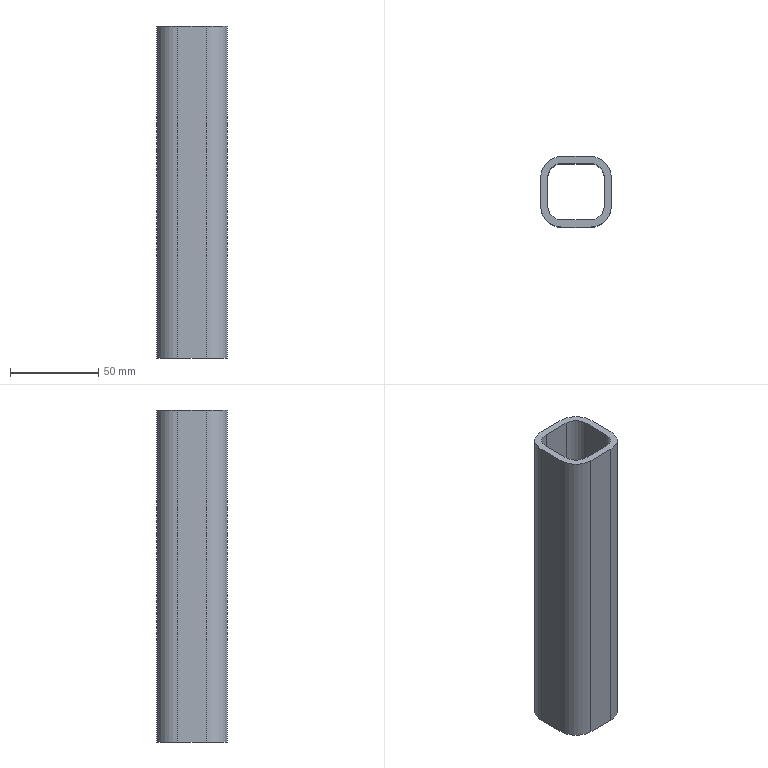Part | SolidWorks | features BaseBody 1 | 1 solid | 18 faces | box 40 x 40 x 188 mm | volume 95378 mm3 | plane 10 | cylinder 8 | commonest cylinder face diameters 16 x4 24 x4
STEP:
#1=CARTESIAN_POINT('',(8.,-20.,0.));
#2=VERTEX_POINT('',#1);
#3=CARTESIAN_POINT('',(20.,-8.,0.));
#4=VERTEX_POINT('',#3);
#5=CARTESIAN_POINT('',(8.,-8.,0.));
#6=DIRECTION('',(0.,0.,1.));
#7=DIRECTION('',(1.,0.,0.));
#8=AXIS2_PLACEMENT_3D('',#5,#6,#7);
#9=CIRCLE('',#8,12.);
#10=EDGE_CURVE('',#2,#4,#9,.T.);
#11=ORIENTED_EDGE('',*,*,#10,.T.);
#12=CARTESIAN_POINT('',(20.,-8.,188.));
#13=VERTEX_POINT('',#12);
#14=CARTESIAN_POINT('',(20.,-8.,0.));
#15=DIRECTION('',(0.,0.,1.));
#16=VECTOR('',#15,1000.);
#17=LINE('',#14,#16);
#18=EDGE_CURVE('',#4,#13,#17,.T.);
#19=ORIENTED_EDGE('',*,*,#18,.T.);
#20=CARTESIAN_POINT('',(8.,-20.,188.));
#21=VERTEX_POINT('',#20);
#22=CARTESIAN_POINT('',(8.,-8.,188.));
#23=DIRECTION('',(0.,0.,-1.));
#24=DIRECTION('',(1.,0.,0.));
#25=AXIS2_PLACEMENT_3D('',#22,#23,#24);
#26=CIRCLE('',#25,12.);
#27=EDGE_CURVE('',#13,#21,#26,.T.);
#28=ORIENTED_EDGE('',*,*,#27,.T.);
#29=CARTESIAN_POINT('',(8.,-20.,0.));
#30=DIRECTION('',(0.,0.,-1.));
#31=VECTOR('',#30,1000.);
#32=LINE('',#29,#31);
#33=EDGE_CURVE('',#21,#2,#32,.T.);
#34=ORIENTED_EDGE('',*,*,#33,.T.);
#35=EDGE_LOOP('',(#11,#19,#28,#34));
#36=FACE_OUTER_BOUND('',#35,.T.);
#37=CARTESIAN_POINT('',(8.,-8.,0.));
#38=DIRECTION('',(0.,0.,1.));
#39=DIRECTION('',(1.,0.,0.));
#40=AXIS2_PLACEMENT_3D('',#37,#38,#39);
#41=CYLINDRICAL_SURFACE('',#40,12.);
#42=ADVANCED_FACE('',(#36),#41,.T.);
#43=CARTESIAN_POINT('',(20.,8.,0.));
#44=VERTEX_POINT('',#43);
#45=CARTESIAN_POINT('',(20.,8.,0.));
#46=DIRECTION('',(0.,1.,0.));
#47=VECTOR('',#46,1000.);
#48=LINE('',#45,#47);
#49=EDGE_CURVE('',#4,#44,#48,.T.);
#50=ORIENTED_EDGE('',*,*,#49,.T.);
#51=CARTESIAN_POINT('',(20.,8.,188.));
#52=VERTEX_POINT('',#51);
#53=CARTESIAN_POINT('',(20.,8.,0.));
#54=DIRECTION('',(0.,0.,1.));
#55=VECTOR('',#54,1000.);
#56=LINE('',#53,#55);
#57=EDGE_CURVE('',#44,#52,#56,.T.);
#58=ORIENTED_EDGE('',*,*,#57,.T.);
#59=CARTESIAN_POINT('',(20.,8.,188.));
#60=DIRECTION('',(0.,-1.,0.));
#61=VECTOR('',#60,1000.);
#62=LINE('',#59,#61);
#63=EDGE_CURVE('',#52,#13,#62,.T.);
#64=ORIENTED_EDGE('',*,*,#63,.T.);
#65=ORIENTED_EDGE('',*,*,#18,.F.);
#66=EDGE_LOOP('',(#50,#58,#64,#65));
#67=FACE_OUTER_BOUND('',#66,.T.);
#68=CARTESIAN_POINT('',(20.,8.,0.));
#69=DIRECTION('',(1.,0.,0.));
#70=DIRECTION('',(0.,1.,0.));
#71=AXIS2_PLACEMENT_3D('',#68,#69,#70);
#72=PLANE('',#71);
#73=ADVANCED_FACE('',(#67),#72,.T.);
#74=CARTESIAN_POINT('',(-16.,8.,0.));
#75=VERTEX_POINT('',#74);
#76=CARTESIAN_POINT('',(-8.,16.,0.));
#77=VERTEX_POINT('',#76);
#78=CARTESIAN_POINT('',(-8.,8.,0.));
#79=DIRECTION('',(0.,0.,-1.));
#80=DIRECTION('',(1.,0.,0.));
#81=AXIS2_PLACEMENT_3D('',#78,#79,#80);
#82=CIRCLE('',#81,8.);
#83=EDGE_CURVE('',#75,#77,#82,.T.);
#84=ORIENTED_EDGE('',*,*,#83,.F.);
#85=CARTESIAN_POINT('',(-16.,-8.,0.));
#86=VERTEX_POINT('',#85);
#87=CARTESIAN_POINT('',(-16.,0.,0.));
#88=DIRECTION('',(0.,1.,0.));
#89=VECTOR('',#88,1000.);
#90=LINE('',#87,#89);
#91=EDGE_CURVE('',#86,#75,#90,.T.);
#92=ORIENTED_EDGE('',*,*,#91,.F.);
#93=CARTESIAN_POINT('',(-8.,-16.,0.));
#94=VERTEX_POINT('',#93);
#95=CARTESIAN_POINT('',(-8.,-8.,0.));
#96=DIRECTION('',(0.,0.,-1.));
#97=DIRECTION('',(1.,0.,0.));
#98=AXIS2_PLACEMENT_3D('',#95,#96,#97);
#99=CIRCLE('',#98,8.);
#100=EDGE_CURVE('',#94,#86,#99,.T.);
#101=ORIENTED_EDGE('',*,*,#100,.F.);
#102=CARTESIAN_POINT('',(8.,-16.,0.));
#103=VERTEX_POINT('',#102);
#104=CARTESIAN_POINT('',(0.,-16.,0.));
#105=DIRECTION('',(-1.,0.,0.));
#106=VECTOR('',#105,1000.);
#107=LINE('',#104,#106);
#108=EDGE_CURVE('',#103,#94,#107,.T.);
#109=ORIENTED_EDGE('',*,*,#108,.F.);
#110=CARTESIAN_POINT('',(16.,-8.,0.));
#111=VERTEX_POINT('',#110);
#112=CARTESIAN_POINT('',(8.,-8.,0.));
#113=DIRECTION('',(0.,0.,-1.));
#114=DIRECTION('',(1.,0.,0.));
#115=AXIS2_PLACEMENT_3D('',#112,#113,#114);
#116=CIRCLE('',#115,8.);
#117=EDGE_CURVE('',#111,#103,#116,.T.);
#118=ORIENTED_EDGE('',*,*,#117,.F.);
#119=CARTESIAN_POINT('',(16.,8.,0.));
#120=VERTEX_POINT('',#119);
#121=CARTESIAN_POINT('',(16.,0.,0.));
#122=DIRECTION('',(0.,-1.,0.));
#123=VECTOR('',#122,1000.);
#124=LINE('',#121,#123);
#125=EDGE_CURVE('',#120,#111,#124,.T.);
#126=ORIENTED_EDGE('',*,*,#125,.F.);
#127=CARTESIAN_POINT('',(8.,16.,0.));
#128=VERTEX_POINT('',#127);
#129=CARTESIAN_POINT('',(8.,8.,0.));
#130=DIRECTION('',(0.,0.,-1.));
#131=DIRECTION('',(1.,0.,0.));
#132=AXIS2_PLACEMENT_3D('',#129,#130,#131);
#133=CIRCLE('',#132,8.);
#134=EDGE_CURVE('',#128,#120,#133,.T.);
#135=ORIENTED_EDGE('',*,*,#134,.F.);
#136=CARTESIAN_POINT('',(0.,16.,0.));
#137=DIRECTION('',(1.,0.,0.));
#138=VECTOR('',#137,1000.);
#139=LINE('',#136,#138);
#140=EDGE_CURVE('',#77,#128,#139,.T.);
#141=ORIENTED_EDGE('',*,*,#140,.F.);
#142=EDGE_LOOP('',(#84,#92,#101,#109,#118,#126,#135,#141));
#143=FACE_BOUND('',#142,.T.);
#144=CARTESIAN_POINT('',(-8.,20.,0.));
#145=VERTEX_POINT('',#144);
#146=CARTESIAN_POINT('',(-20.,8.,0.));
#147=VERTEX_POINT('',#146);
#148=CARTESIAN_POINT('',(-8.,8.,0.));
#149=DIRECTION('',(0.,0.,1.));
#150=DIRECTION('',(1.,0.,0.));
#151=AXIS2_PLACEMENT_3D('',#148,#149,#150);
#152=CIRCLE('',#151,12.);
#153=EDGE_CURVE('',#145,#147,#152,.T.);
#154=ORIENTED_EDGE('',*,*,#153,.F.);
#155=CARTESIAN_POINT('',(8.,20.,0.));
#156=VERTEX_POINT('',#155);
#157=CARTESIAN_POINT('',(0.,20.,0.));
#158=DIRECTION('',(-1.,0.,0.));
#159=VECTOR('',#158,1000.);
#160=LINE('',#157,#159);
#161=EDGE_CURVE('',#156,#145,#160,.T.);
#162=ORIENTED_EDGE('',*,*,#161,.F.);
#163=CARTESIAN_POINT('',(8.,8.,0.));
#164=DIRECTION('',(0.,0.,1.));
#165=DIRECTION('',(1.,0.,0.));
#166=AXIS2_PLACEMENT_3D('',#163,#164,#165);
#167=CIRCLE('',#166,12.);
#168=EDGE_CURVE('',#44,#156,#167,.T.);
#169=ORIENTED_EDGE('',*,*,#168,.F.);
#170=ORIENTED_EDGE('',*,*,#49,.F.);
#171=ORIENTED_EDGE('',*,*,#10,.F.);
#172=CARTESIAN_POINT('',(-8.,-20.,0.));
#173=VERTEX_POINT('',#172);
#174=CARTESIAN_POINT('',(0.,-20.,0.));
#175=DIRECTION('',(1.,0.,0.));
#176=VECTOR('',#175,1000.);
#177=LINE('',#174,#176);
#178=EDGE_CURVE('',#173,#2,#177,.T.);
#179=ORIENTED_EDGE('',*,*,#178,.F.);
#180=CARTESIAN_POINT('',(-20.,-8.,0.));
#181=VERTEX_POINT('',#180);
#182=CARTESIAN_POINT('',(-8.,-8.,0.));
#183=DIRECTION('',(0.,0.,1.));
#184=DIRECTION('',(1.,0.,0.));
#185=AXIS2_PLACEMENT_3D('',#182,#183,#184);
#186=CIRCLE('',#185,12.);
#187=EDGE_CURVE('',#181,#173,#186,.T.);
#188=ORIENTED_EDGE('',*,*,#187,.F.);
#189=CARTESIAN_POINT('',(-20.,0.,0.));
#190=DIRECTION('',(0.,-1.,0.));
#191=VECTOR('',#190,1000.);
#192=LINE('',#189,#191);
#193=EDGE_CURVE('',#147,#181,#192,.T.);
#194=ORIENTED_EDGE('',*,*,#193,.F.);
#195=EDGE_LOOP('',(#154,#162,#169,#170,#171,#179,#188,#194));
#196=FACE_OUTER_BOUND('',#195,.T.);
#197=CARTESIAN_POINT('',(0.,0.,0.));
#198=DIRECTION('',(0.,0.,1.));
#199=DIRECTION('',(1.,0.,0.));
#200=AXIS2_PLACEMENT_3D('',#197,#198,#199);
#201=PLANE('',#200);
#202=ADVANCED_FACE('',(#143,#196),#201,.F.);
#203=ORIENTED_EDGE('',*,*,#178,.T.);
#204=ORIENTED_EDGE('',*,*,#33,.F.);
#205=CARTESIAN_POINT('',(-8.,-20.,188.));
#206=VERTEX_POINT('',#205);
#207=CARTESIAN_POINT('',(8.,-20.,188.));
#208=DIRECTION('',(-1.,0.,0.));
#209=VECTOR('',#208,1000.);
#210=LINE('',#207,#209);
#211=EDGE_CURVE('',#21,#206,#210,.T.);
#212=ORIENTED_EDGE('',*,*,#211,.T.);
#213=CARTESIAN_POINT('',(-8.,-20.,0.));
#214=DIRECTION('',(0.,0.,-1.));
#215=VECTOR('',#214,1000.);
#216=LINE('',#213,#215);
#217=EDGE_CURVE('',#206,#173,#216,.T.);
#218=ORIENTED_EDGE('',*,*,#217,.T.);
#219=EDGE_LOOP('',(#203,#204,#212,#218));
#220=FACE_OUTER_BOUND('',#219,.T.);
#221=CARTESIAN_POINT('',(8.,-20.,0.));
#222=DIRECTION('',(0.,-1.,0.));
#223=DIRECTION('',(1.,0.,0.));
#224=AXIS2_PLACEMENT_3D('',#221,#222,#223);
#225=PLANE('',#224);
#226=ADVANCED_FACE('',(#220),#225,.T.);
#227=CARTESIAN_POINT('',(-16.,-8.,188.));
#228=VERTEX_POINT('',#227);
#229=CARTESIAN_POINT('',(-16.,8.,188.));
#230=VERTEX_POINT('',#229);
#231=CARTESIAN_POINT('',(-16.,0.,188.));
#232=DIRECTION('',(0.,1.,0.));
#233=VECTOR('',#232,1000.);
#234=LINE('',#231,#233);
#235=EDGE_CURVE('',#228,#230,#234,.T.);
#236=ORIENTED_EDGE('',*,*,#235,.T.);
#237=CARTESIAN_POINT('',(-8.,16.,188.));
#238=VERTEX_POINT('',#237);
#239=CARTESIAN_POINT('',(-8.,8.,188.));
#240=DIRECTION('',(0.,0.,-1.));
#241=DIRECTION('',(1.,0.,0.));
#242=AXIS2_PLACEMENT_3D('',#239,#240,#241);
#243=CIRCLE('',#242,8.);
#244=EDGE_CURVE('',#230,#238,#243,.T.);
#245=ORIENTED_EDGE('',*,*,#244,.T.);
#246=CARTESIAN_POINT('',(8.,16.,188.));
#247=VERTEX_POINT('',#246);
#248=CARTESIAN_POINT('',(0.,16.,188.));
#249=DIRECTION('',(1.,0.,0.));
#250=VECTOR('',#249,1000.);
#251=LINE('',#248,#250);
#252=EDGE_CURVE('',#238,#247,#251,.T.);
#253=ORIENTED_EDGE('',*,*,#252,.T.);
#254=CARTESIAN_POINT('',(16.,8.,188.));
#255=VERTEX_POINT('',#254);
#256=CARTESIAN_POINT('',(8.,8.,188.));
#257=DIRECTION('',(0.,0.,-1.));
#258=DIRECTION('',(1.,0.,0.));
#259=AXIS2_PLACEMENT_3D('',#256,#257,#258);
#260=CIRCLE('',#259,8.);
#261=EDGE_CURVE('',#247,#255,#260,.T.);
#262=ORIENTED_EDGE('',*,*,#261,.T.);
#263=CARTESIAN_POINT('',(16.,-8.,188.));
#264=VERTEX_POINT('',#263);
#265=CARTESIAN_POINT('',(16.,0.,188.));
#266=DIRECTION('',(0.,-1.,0.));
#267=VECTOR('',#266,1000.);
#268=LINE('',#265,#267);
#269=EDGE_CURVE('',#255,#264,#268,.T.);
#270=ORIENTED_EDGE('',*,*,#269,.T.);
#271=CARTESIAN_POINT('',(8.,-16.,188.));
#272=VERTEX_POINT('',#271);
#273=CARTESIAN_POINT('',(8.,-8.,188.));
#274=DIRECTION('',(0.,0.,-1.));
#275=DIRECTION('',(1.,0.,0.));
#276=AXIS2_PLACEMENT_3D('',#273,#274,#275);
#277=CIRCLE('',#276,8.);
#278=EDGE_CURVE('',#264,#272,#277,.T.);
#279=ORIENTED_EDGE('',*,*,#278,.T.);
#280=CARTESIAN_POINT('',(-8.,-16.,188.));
#281=VERTEX_POINT('',#280);
#282=CARTESIAN_POINT('',(0.,-16.,188.));
#283=DIRECTION('',(-1.,0.,0.));
#284=VECTOR('',#283,1000.);
#285=LINE('',#282,#284);
#286=EDGE_CURVE('',#272,#281,#285,.T.);
#287=ORIENTED_EDGE('',*,*,#286,.T.);
#288=CARTESIAN_POINT('',(-8.,-8.,188.));
#289=DIRECTION('',(0.,0.,-1.));
#290=DIRECTION('',(1.,0.,0.));
#291=AXIS2_PLACEMENT_3D('',#288,#289,#290);
#292=CIRCLE('',#291,8.);
#293=EDGE_CURVE('',#281,#228,#292,.T.);
#294=ORIENTED_EDGE('',*,*,#293,.T.);
#295=EDGE_LOOP('',(#236,#245,#253,#262,#270,#279,#287,#294));
#296=FACE_BOUND('',#295,.T.);
#297=CARTESIAN_POINT('',(8.,20.,188.));
#298=VERTEX_POINT('',#297);
#299=CARTESIAN_POINT('',(-8.,20.,188.));
#300=VERTEX_POINT('',#299);
#301=CARTESIAN_POINT('',(0.,20.,188.));
#302=DIRECTION('',(-1.,0.,0.));
#303=VECTOR('',#302,1000.);
#304=LINE('',#301,#303);
#305=EDGE_CURVE('',#298,#300,#304,.T.);
#306=ORIENTED_EDGE('',*,*,#305,.T.);
#307=CARTESIAN_POINT('',(-20.,8.,188.));
#308=VERTEX_POINT('',#307);
#309=CARTESIAN_POINT('',(-8.,8.,188.));
#310=DIRECTION('',(0.,0.,1.));
#311=DIRECTION('',(1.,0.,0.));
#312=AXIS2_PLACEMENT_3D('',#309,#310,#311);
#313=CIRCLE('',#312,12.);
#314=EDGE_CURVE('',#300,#308,#313,.T.);
#315=ORIENTED_EDGE('',*,*,#314,.T.);
#316=CARTESIAN_POINT('',(-20.,-8.,188.));
#317=VERTEX_POINT('',#316);
#318=CARTESIAN_POINT('',(-20.,0.,188.));
#319=DIRECTION('',(0.,-1.,0.));
#320=VECTOR('',#319,1000.);
#321=LINE('',#318,#320);
#322=EDGE_CURVE('',#308,#317,#321,.T.);
#323=ORIENTED_EDGE('',*,*,#322,.T.);
#324=CARTESIAN_POINT('',(-8.,-8.,188.));
#325=DIRECTION('',(0.,0.,1.));
#326=DIRECTION('',(1.,0.,0.));
#327=AXIS2_PLACEMENT_3D('',#324,#325,#326);
#328=CIRCLE('',#327,12.);
#329=EDGE_CURVE('',#317,#206,#328,.T.);
#330=ORIENTED_EDGE('',*,*,#329,.T.);
#331=ORIENTED_EDGE('',*,*,#211,.F.);
#332=ORIENTED_EDGE('',*,*,#27,.F.);
#333=ORIENTED_EDGE('',*,*,#63,.F.);
#334=CARTESIAN_POINT('',(8.,8.,188.));
#335=DIRECTION('',(0.,0.,1.));
#336=DIRECTION('',(1.,0.,0.));
#337=AXIS2_PLACEMENT_3D('',#334,#335,#336);
#338=CIRCLE('',#337,12.);
#339=EDGE_CURVE('',#52,#298,#338,.T.);
#340=ORIENTED_EDGE('',*,*,#339,.T.);
#341=EDGE_LOOP('',(#306,#315,#323,#330,#331,#332,#333,#340));
#342=FACE_OUTER_BOUND('',#341,.T.);
#343=CARTESIAN_POINT('',(0.,0.,188.));
#344=DIRECTION('',(0.,0.,1.));
#345=DIRECTION('',(1.,0.,0.));
#346=AXIS2_PLACEMENT_3D('',#343,#344,#345);
#347=PLANE('',#346);
#348=ADVANCED_FACE('',(#296,#342),#347,.T.);
#349=ORIENTED_EDGE('',*,*,#168,.T.);
#350=CARTESIAN_POINT('',(8.,20.,0.));
#351=DIRECTION('',(0.,0.,1.));
#352=VECTOR('',#351,1000.);
#353=LINE('',#350,#352);
#354=EDGE_CURVE('',#156,#298,#353,.T.);
#355=ORIENTED_EDGE('',*,*,#354,.T.);
#356=ORIENTED_EDGE('',*,*,#339,.F.);
#357=ORIENTED_EDGE('',*,*,#57,.F.);
#358=EDGE_LOOP('',(#349,#355,#356,#357));
#359=FACE_OUTER_BOUND('',#358,.T.);
#360=CARTESIAN_POINT('',(8.,8.,0.));
#361=DIRECTION('',(0.,0.,1.));
#362=DIRECTION('',(1.,0.,0.));
#363=AXIS2_PLACEMENT_3D('',#360,#361,#362);
#364=CYLINDRICAL_SURFACE('',#363,12.);
#365=ADVANCED_FACE('',(#359),#364,.T.);
#366=CARTESIAN_POINT('',(-8.,16.,0.));
#367=DIRECTION('',(0.,0.,1.));
#368=VECTOR('',#367,1000.);
#369=LINE('',#366,#368);
#370=EDGE_CURVE('',#77,#238,#369,.T.);
#371=ORIENTED_EDGE('',*,*,#370,.F.);
#372=ORIENTED_EDGE('',*,*,#140,.T.);
#373=CARTESIAN_POINT('',(8.,16.,0.));
#374=DIRECTION('',(0.,0.,-1.));
#375=VECTOR('',#374,1000.);
#376=LINE('',#373,#375);
#377=EDGE_CURVE('',#247,#128,#376,.T.);
#378=ORIENTED_EDGE('',*,*,#377,.F.);
#379=ORIENTED_EDGE('',*,*,#252,.F.);
#380=EDGE_LOOP('',(#371,#372,#378,#379));
#381=FACE_OUTER_BOUND('',#380,.T.);
#382=CARTESIAN_POINT('',(-8.,16.,0.));
#383=DIRECTION('',(0.,1.,0.));
#384=DIRECTION('',(-1.,0.,0.));
#385=AXIS2_PLACEMENT_3D('',#382,#383,#384);
#386=PLANE('',#385);
#387=ADVANCED_FACE('',(#381),#386,.F.);
#388=CARTESIAN_POINT('',(-16.,8.,0.));
#389=DIRECTION('',(0.,0.,1.));
#390=VECTOR('',#389,1000.);
#391=LINE('',#388,#390);
#392=EDGE_CURVE('',#75,#230,#391,.T.);
#393=ORIENTED_EDGE('',*,*,#392,.F.);
#394=ORIENTED_EDGE('',*,*,#83,.T.);
#395=ORIENTED_EDGE('',*,*,#370,.T.);
#396=ORIENTED_EDGE('',*,*,#244,.F.);
#397=EDGE_LOOP('',(#393,#394,#395,#396));
#398=FACE_OUTER_BOUND('',#397,.T.);
#399=CARTESIAN_POINT('',(-8.,8.,0.));
#400=DIRECTION('',(0.,0.,1.));
#401=DIRECTION('',(1.,0.,0.));
#402=AXIS2_PLACEMENT_3D('',#399,#400,#401);
#403=CYLINDRICAL_SURFACE('',#402,8.);
#404=ADVANCED_FACE('',(#398),#403,.F.);
#405=CARTESIAN_POINT('',(-16.,-8.,0.));
#406=DIRECTION('',(0.,0.,1.));
#407=VECTOR('',#406,1000.);
#408=LINE('',#405,#407);
#409=EDGE_CURVE('',#86,#228,#408,.T.);
#410=ORIENTED_EDGE('',*,*,#409,.F.);
#411=ORIENTED_EDGE('',*,*,#91,.T.);
#412=ORIENTED_EDGE('',*,*,#392,.T.);
#413=ORIENTED_EDGE('',*,*,#235,.F.);
#414=EDGE_LOOP('',(#410,#411,#412,#413));
#415=FACE_OUTER_BOUND('',#414,.T.);
#416=CARTESIAN_POINT('',(-16.,-8.,0.));
#417=DIRECTION('',(-1.,0.,0.));
#418=DIRECTION('',(0.,-1.,0.));
#419=AXIS2_PLACEMENT_3D('',#416,#417,#418);
#420=PLANE('',#419);
#421=ADVANCED_FACE('',(#415),#420,.F.);
#422=CARTESIAN_POINT('',(-8.,-16.,0.));
#423=DIRECTION('',(0.,0.,1.));
#424=VECTOR('',#423,1000.);
#425=LINE('',#422,#424);
#426=EDGE_CURVE('',#94,#281,#425,.T.);
#427=ORIENTED_EDGE('',*,*,#426,.F.);
#428=ORIENTED_EDGE('',*,*,#100,.T.);
#429=ORIENTED_EDGE('',*,*,#409,.T.);
#430=ORIENTED_EDGE('',*,*,#293,.F.);
#431=EDGE_LOOP('',(#427,#428,#429,#430));
#432=FACE_OUTER_BOUND('',#431,.T.);
#433=CARTESIAN_POINT('',(-8.,-8.,0.));
#434=DIRECTION('',(0.,0.,1.));
#435=DIRECTION('',(1.,0.,0.));
#436=AXIS2_PLACEMENT_3D('',#433,#434,#435);
#437=CYLINDRICAL_SURFACE('',#436,8.);
#438=ADVANCED_FACE('',(#432),#437,.F.);
#439=CARTESIAN_POINT('',(8.,-16.,0.));
#440=DIRECTION('',(0.,0.,1.));
#441=VECTOR('',#440,1000.);
#442=LINE('',#439,#441);
#443=EDGE_CURVE('',#103,#272,#442,.T.);
#444=ORIENTED_EDGE('',*,*,#443,.F.);
#445=ORIENTED_EDGE('',*,*,#108,.T.);
#446=ORIENTED_EDGE('',*,*,#426,.T.);
#447=ORIENTED_EDGE('',*,*,#286,.F.);
#448=EDGE_LOOP('',(#444,#445,#446,#447));
#449=FACE_OUTER_BOUND('',#448,.T.);
#450=CARTESIAN_POINT('',(8.,-16.,0.));
#451=DIRECTION('',(0.,-1.,0.));
#452=DIRECTION('',(1.,0.,0.));
#453=AXIS2_PLACEMENT_3D('',#450,#451,#452);
#454=PLANE('',#453);
#455=ADVANCED_FACE('',(#449),#454,.F.);
#456=CARTESIAN_POINT('',(16.,-8.,0.));
#457=DIRECTION('',(0.,0.,1.));
#458=VECTOR('',#457,1000.);
#459=LINE('',#456,#458);
#460=EDGE_CURVE('',#111,#264,#459,.T.);
#461=ORIENTED_EDGE('',*,*,#460,.F.);
#462=ORIENTED_EDGE('',*,*,#117,.T.);
#463=ORIENTED_EDGE('',*,*,#443,.T.);
#464=ORIENTED_EDGE('',*,*,#278,.F.);
#465=EDGE_LOOP('',(#461,#462,#463,#464));
#466=FACE_OUTER_BOUND('',#465,.T.);
#467=CARTESIAN_POINT('',(8.,-8.,0.));
#468=DIRECTION('',(0.,0.,1.));
#469=DIRECTION('',(1.,0.,0.));
#470=AXIS2_PLACEMENT_3D('',#467,#468,#469);
#471=CYLINDRICAL_SURFACE('',#470,8.);
#472=ADVANCED_FACE('',(#466),#471,.F.);
#473=CARTESIAN_POINT('',(16.,8.,0.));
#474=DIRECTION('',(0.,0.,1.));
#475=VECTOR('',#474,1000.);
#476=LINE('',#473,#475);
#477=EDGE_CURVE('',#120,#255,#476,.T.);
#478=ORIENTED_EDGE('',*,*,#477,.F.);
#479=ORIENTED_EDGE('',*,*,#125,.T.);
#480=ORIENTED_EDGE('',*,*,#460,.T.);
#481=ORIENTED_EDGE('',*,*,#269,.F.);
#482=EDGE_LOOP('',(#478,#479,#480,#481));
#483=FACE_OUTER_BOUND('',#482,.T.);
#484=CARTESIAN_POINT('',(16.,8.,0.));
#485=DIRECTION('',(1.,0.,0.));
#486=DIRECTION('',(0.,0.,-1.));
#487=AXIS2_PLACEMENT_3D('',#484,#485,#486);
#488=PLANE('',#487);
#489=ADVANCED_FACE('',(#483),#488,.F.);
#490=ORIENTED_EDGE('',*,*,#377,.T.);
#491=ORIENTED_EDGE('',*,*,#134,.T.);
#492=ORIENTED_EDGE('',*,*,#477,.T.);
#493=ORIENTED_EDGE('',*,*,#261,.F.);
#494=EDGE_LOOP('',(#490,#491,#492,#493));
#495=FACE_OUTER_BOUND('',#494,.T.);
#496=CARTESIAN_POINT('',(8.,8.,0.));
#497=DIRECTION('',(0.,0.,1.));
#498=DIRECTION('',(1.,0.,0.));
#499=AXIS2_PLACEMENT_3D('',#496,#497,#498);
#500=CYLINDRICAL_SURFACE('',#499,8.);
#501=ADVANCED_FACE('',(#495),#500,.F.);
#502=ORIENTED_EDGE('',*,*,#193,.T.);
#503=CARTESIAN_POINT('',(-20.,-8.,0.));
#504=DIRECTION('',(0.,0.,1.));
#505=VECTOR('',#504,1000.);
#506=LINE('',#503,#505);
#507=EDGE_CURVE('',#181,#317,#506,.T.);
#508=ORIENTED_EDGE('',*,*,#507,.T.);
#509=ORIENTED_EDGE('',*,*,#322,.F.);
#510=CARTESIAN_POINT('',(-20.,8.,0.));
#511=DIRECTION('',(0.,0.,-1.));
#512=VECTOR('',#511,1000.);
#513=LINE('',#510,#512);
#514=EDGE_CURVE('',#308,#147,#513,.T.);
#515=ORIENTED_EDGE('',*,*,#514,.T.);
#516=EDGE_LOOP('',(#502,#508,#509,#515));
#517=FACE_OUTER_BOUND('',#516,.T.);
#518=CARTESIAN_POINT('',(-20.,-8.,0.));
#519=DIRECTION('',(-1.,0.,0.));
#520=DIRECTION('',(0.,-1.,0.));
#521=AXIS2_PLACEMENT_3D('',#518,#519,#520);
#522=PLANE('',#521);
#523=ADVANCED_FACE('',(#517),#522,.T.);
#524=ORIENTED_EDGE('',*,*,#153,.T.);
#525=ORIENTED_EDGE('',*,*,#514,.F.);
#526=ORIENTED_EDGE('',*,*,#314,.F.);
#527=CARTESIAN_POINT('',(-8.,20.,0.));
#528=DIRECTION('',(0.,0.,-1.));
#529=VECTOR('',#528,1000.);
#530=LINE('',#527,#529);
#531=EDGE_CURVE('',#300,#145,#530,.T.);
#532=ORIENTED_EDGE('',*,*,#531,.T.);
#533=EDGE_LOOP('',(#524,#525,#526,#532));
#534=FACE_OUTER_BOUND('',#533,.T.);
#535=CARTESIAN_POINT('',(-8.,8.,0.));
#536=DIRECTION('',(0.,0.,1.));
#537=DIRECTION('',(1.,0.,0.));
#538=AXIS2_PLACEMENT_3D('',#535,#536,#537);
#539=CYLINDRICAL_SURFACE('',#538,12.);
#540=ADVANCED_FACE('',(#534),#539,.T.);
#541=ORIENTED_EDGE('',*,*,#161,.T.);
#542=ORIENTED_EDGE('',*,*,#531,.F.);
#543=ORIENTED_EDGE('',*,*,#305,.F.);
#544=ORIENTED_EDGE('',*,*,#354,.F.);
#545=EDGE_LOOP('',(#541,#542,#543,#544));
#546=FACE_OUTER_BOUND('',#545,.T.);
#547=CARTESIAN_POINT('',(-8.,20.,0.));
#548=DIRECTION('',(0.,1.,0.));
#549=DIRECTION('',(0.,0.,1.));
#550=AXIS2_PLACEMENT_3D('',#547,#548,#549);
#551=PLANE('',#550);
#552=ADVANCED_FACE('',(#546),#551,.T.);
#553=ORIENTED_EDGE('',*,*,#187,.T.);
#554=ORIENTED_EDGE('',*,*,#217,.F.);
#555=ORIENTED_EDGE('',*,*,#329,.F.);
#556=ORIENTED_EDGE('',*,*,#507,.F.);
#557=EDGE_LOOP('',(#553,#554,#555,#556));
#558=FACE_OUTER_BOUND('',#557,.T.);
#559=CARTESIAN_POINT('',(-8.,-8.,0.));
#560=DIRECTION('',(0.,0.,1.));
#561=DIRECTION('',(1.,0.,0.));
#562=AXIS2_PLACEMENT_3D('',#559,#560,#561);
#563=CYLINDRICAL_SURFACE('',#562,12.);
#564=ADVANCED_FACE('',(#558),#563,.T.);
#565=CLOSED_SHELL('',(#42,#73,#202,#226,#348,#365,#387,#404,#421,#438,#455,#472,#489,#501,#523,#540,#552,#564));
#566=MANIFOLD_SOLID_BREP('',#565);
#567=CARTESIAN_POINT('',(0.,0.,0.));
#568=DIRECTION('',(0.,0.,1.));
#569=DIRECTION('',(1.,0.,0.));
#570=AXIS2_PLACEMENT_3D('',#567,#568,#569);
#571=(LENGTH_UNIT()NAMED_UNIT(*)SI_UNIT(.MILLI.,.METRE.));
#572=UNCERTAINTY_MEASURE_WITH_UNIT(LENGTH_MEASURE(0.00001),#571,'','');
#573=(NAMED_UNIT(*)PLANE_ANGLE_UNIT()SI_UNIT($,.RADIAN.));
#574=(NAMED_UNIT(*)SI_UNIT($,.STERADIAN.)SOLID_ANGLE_UNIT());
#575=(GEOMETRIC_REPRESENTATION_CONTEXT(3)GLOBAL_UNCERTAINTY_ASSIGNED_CONTEXT((#572))GLOBAL_UNIT_ASSIGNED_CONTEXT((#571,#573,#574))REPRESENTATION_CONTEXT('',''));
#576=ADVANCED_BREP_SHAPE_REPRESENTATION('',(#566,#570),#575);